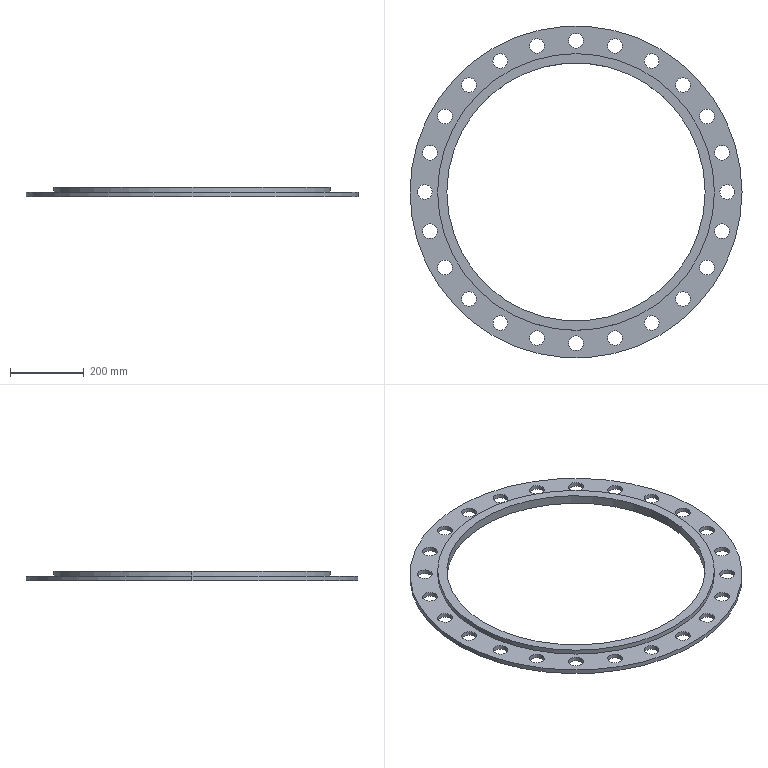Part | SolidWorks | features ICE 3, Extrusion 1 | 1 solid | 57 faces | box 900 x 900 x 25 mm | volume 3394255 mm3 | cylinder 54 | plane 3 | commonest cylinder face diameters 40 x48 700 x2 750 x2 900 x2